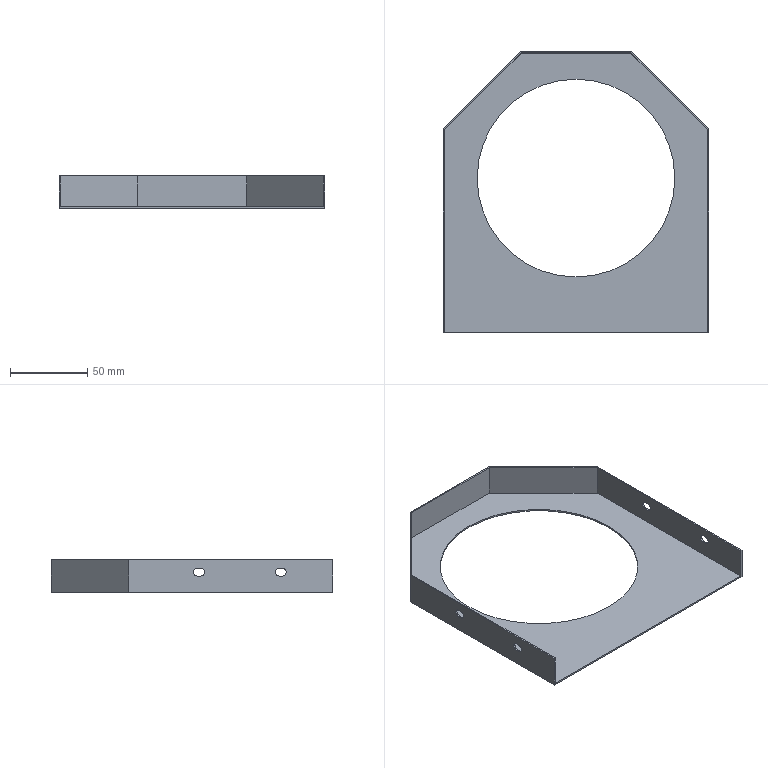Part | SolidWorks | features BaseBody 1 | 1 solid | 32 faces | box 172 x 182 x 21 mm | volume 25333 mm3 | plane 22 | cylinder 10 | commonest cylinder face diameters 5 x8 128 x2
STEP:
#1=CARTESIAN_POINT('',(150.,-82.,1.));
#2=VERTEX_POINT('',#1);
#3=CARTESIAN_POINT('',(22.,-82.,1.));
#4=VERTEX_POINT('',#3);
#5=CARTESIAN_POINT('',(86.,-82.,1.));
#6=DIRECTION('',(0.,0.,-1.));
#7=DIRECTION('',(-1.,0.,0.));
#8=AXIS2_PLACEMENT_3D('',#5,#6,#7);
#9=CIRCLE('',#8,64.);
#10=EDGE_CURVE('',#2,#4,#9,.T.);
#11=ORIENTED_EDGE('',*,*,#10,.F.);
#12=CARTESIAN_POINT('',(150.,-82.,0.));
#13=VERTEX_POINT('',#12);
#14=CARTESIAN_POINT('',(150.,-82.,1.));
#15=DIRECTION('',(0.,0.,-1.));
#16=VECTOR('',#15,1000.);
#17=LINE('',#14,#16);
#18=EDGE_CURVE('',#2,#13,#17,.T.);
#19=ORIENTED_EDGE('',*,*,#18,.T.);
#20=CARTESIAN_POINT('',(22.,-82.,0.));
#21=VERTEX_POINT('',#20);
#22=CARTESIAN_POINT('',(86.,-82.,0.));
#23=DIRECTION('',(0.,0.,-1.));
#24=DIRECTION('',(-1.,0.,0.));
#25=AXIS2_PLACEMENT_3D('',#22,#23,#24);
#26=CIRCLE('',#25,64.);
#27=EDGE_CURVE('',#13,#21,#26,.T.);
#28=ORIENTED_EDGE('',*,*,#27,.T.);
#29=CARTESIAN_POINT('',(22.,-82.,1.));
#30=DIRECTION('',(0.,0.,-1.));
#31=VECTOR('',#30,1000.);
#32=LINE('',#29,#31);
#33=EDGE_CURVE('',#4,#21,#32,.T.);
#34=ORIENTED_EDGE('',*,*,#33,.F.);
#35=EDGE_LOOP('',(#11,#19,#28,#34));
#36=FACE_OUTER_BOUND('',#35,.T.);
#37=CARTESIAN_POINT('',(86.,-82.,1.));
#38=DIRECTION('',(0.,0.,-1.));
#39=DIRECTION('',(-1.,0.,0.));
#40=AXIS2_PLACEMENT_3D('',#37,#38,#39);
#41=CYLINDRICAL_SURFACE('',#40,64.);
#42=ADVANCED_FACE('',(#36),#41,.F.);
#43=CARTESIAN_POINT('',(86.,-82.,0.));
#44=DIRECTION('',(0.,0.,-1.));
#45=DIRECTION('',(-1.,0.,0.));
#46=AXIS2_PLACEMENT_3D('',#43,#44,#45);
#47=CIRCLE('',#46,64.);
#48=EDGE_CURVE('',#21,#13,#47,.T.);
#49=ORIENTED_EDGE('',*,*,#48,.F.);
#50=ORIENTED_EDGE('',*,*,#27,.F.);
#51=EDGE_LOOP('',(#49,#50));
#52=FACE_BOUND('',#51,.T.);
#53=CARTESIAN_POINT('',(0.,-182.,0.));
#54=VERTEX_POINT('',#53);
#55=CARTESIAN_POINT('',(172.,-182.,0.));
#56=VERTEX_POINT('',#55);
#57=CARTESIAN_POINT('',(0.,-182.,0.));
#58=DIRECTION('',(1.,0.,0.));
#59=VECTOR('',#58,1000.);
#60=LINE('',#57,#59);
#61=EDGE_CURVE('',#54,#56,#60,.T.);
#62=ORIENTED_EDGE('',*,*,#61,.F.);
#63=CARTESIAN_POINT('',(0.,-50.,0.));
#64=VERTEX_POINT('',#63);
#65=CARTESIAN_POINT('',(0.,0.,0.));
#66=DIRECTION('',(0.,-1.,0.));
#67=VECTOR('',#66,1000.);
#68=LINE('',#65,#67);
#69=EDGE_CURVE('',#64,#54,#68,.T.);
#70=ORIENTED_EDGE('',*,*,#69,.F.);
#71=CARTESIAN_POINT('',(50.,0.,0.));
#72=VERTEX_POINT('',#71);
#73=CARTESIAN_POINT('',(50.,0.,0.));
#74=DIRECTION('',(-0.7071,-0.7071,0.));
#75=VECTOR('',#74,1000.);
#76=LINE('',#73,#75);
#77=EDGE_CURVE('',#72,#64,#76,.T.);
#78=ORIENTED_EDGE('',*,*,#77,.F.);
#79=CARTESIAN_POINT('',(122.,0.,0.));
#80=VERTEX_POINT('',#79);
#81=CARTESIAN_POINT('',(0.,0.,0.));
#82=DIRECTION('',(-1.,0.,0.));
#83=VECTOR('',#82,1000.);
#84=LINE('',#81,#83);
#85=EDGE_CURVE('',#80,#72,#84,.T.);
#86=ORIENTED_EDGE('',*,*,#85,.F.);
#87=CARTESIAN_POINT('',(172.,-50.,0.));
#88=VERTEX_POINT('',#87);
#89=CARTESIAN_POINT('',(172.,-50.,0.));
#90=DIRECTION('',(-0.7071,0.7071,0.));
#91=VECTOR('',#90,1000.);
#92=LINE('',#89,#91);
#93=EDGE_CURVE('',#88,#80,#92,.T.);
#94=ORIENTED_EDGE('',*,*,#93,.F.);
#95=CARTESIAN_POINT('',(172.,0.,0.));
#96=DIRECTION('',(0.,1.,0.));
#97=VECTOR('',#96,1000.);
#98=LINE('',#95,#97);
#99=EDGE_CURVE('',#56,#88,#98,.T.);
#100=ORIENTED_EDGE('',*,*,#99,.F.);
#101=EDGE_LOOP('',(#62,#70,#78,#86,#94,#100));
#102=FACE_OUTER_BOUND('',#101,.T.);
#103=CARTESIAN_POINT('',(0.,0.,0.));
#104=DIRECTION('',(0.,0.,1.));
#105=DIRECTION('',(1.,0.,0.));
#106=AXIS2_PLACEMENT_3D('',#103,#104,#105);
#107=PLANE('',#106);
#108=ADVANCED_FACE('',(#52,#102),#107,.F.);
#109=ORIENTED_EDGE('',*,*,#18,.F.);
#110=CARTESIAN_POINT('',(86.,-82.,1.));
#111=DIRECTION('',(0.,0.,-1.));
#112=DIRECTION('',(-1.,0.,0.));
#113=AXIS2_PLACEMENT_3D('',#110,#111,#112);
#114=CIRCLE('',#113,64.);
#115=EDGE_CURVE('',#4,#2,#114,.T.);
#116=ORIENTED_EDGE('',*,*,#115,.F.);
#117=ORIENTED_EDGE('',*,*,#33,.T.);
#118=ORIENTED_EDGE('',*,*,#48,.T.);
#119=EDGE_LOOP('',(#109,#116,#117,#118));
#120=FACE_OUTER_BOUND('',#119,.T.);
#121=CARTESIAN_POINT('',(86.,-82.,1.));
#122=DIRECTION('',(0.,0.,-1.));
#123=DIRECTION('',(-1.,0.,0.));
#124=AXIS2_PLACEMENT_3D('',#121,#122,#123);
#125=CYLINDRICAL_SURFACE('',#124,64.);
#126=ADVANCED_FACE('',(#120),#125,.F.);
#127=CARTESIAN_POINT('',(172.,-94.5,10.5));
#128=VERTEX_POINT('',#127);
#129=CARTESIAN_POINT('',(172.,-94.5,15.5));
#130=VERTEX_POINT('',#129);
#131=CARTESIAN_POINT('',(172.,-94.5,13.));
#132=DIRECTION('',(1.,0.,0.));
#133=DIRECTION('',(0.,0.,1.));
#134=AXIS2_PLACEMENT_3D('',#131,#132,#133);
#135=CIRCLE('',#134,2.5);
#136=EDGE_CURVE('',#128,#130,#135,.T.);
#137=ORIENTED_EDGE('',*,*,#136,.F.);
#138=CARTESIAN_POINT('',(172.,-96.5,10.5));
#139=VERTEX_POINT('',#138);
#140=CARTESIAN_POINT('',(172.,-50.,10.5));
#141=DIRECTION('',(0.,1.,0.));
#142=VECTOR('',#141,1000.);
#143=LINE('',#140,#142);
#144=EDGE_CURVE('',#139,#128,#143,.T.);
#145=ORIENTED_EDGE('',*,*,#144,.F.);
#146=CARTESIAN_POINT('',(172.,-96.5,15.5));
#147=VERTEX_POINT('',#146);
#148=CARTESIAN_POINT('',(172.,-96.5,13.));
#149=DIRECTION('',(1.,0.,0.));
#150=DIRECTION('',(0.,0.,1.));
#151=AXIS2_PLACEMENT_3D('',#148,#149,#150);
#152=CIRCLE('',#151,2.5);
#153=EDGE_CURVE('',#147,#139,#152,.T.);
#154=ORIENTED_EDGE('',*,*,#153,.F.);
#155=CARTESIAN_POINT('',(172.,-50.,15.5));
#156=DIRECTION('',(0.,-1.,0.));
#157=VECTOR('',#156,1000.);
#158=LINE('',#155,#157);
#159=EDGE_CURVE('',#130,#147,#158,.T.);
#160=ORIENTED_EDGE('',*,*,#159,.F.);
#161=EDGE_LOOP('',(#137,#145,#154,#160));
#162=FACE_BOUND('',#161,.T.);
#163=CARTESIAN_POINT('',(172.,-147.5,10.5));
#164=VERTEX_POINT('',#163);
#165=CARTESIAN_POINT('',(172.,-147.5,15.5));
#166=VERTEX_POINT('',#165);
#167=CARTESIAN_POINT('',(172.,-147.5,13.));
#168=DIRECTION('',(1.,0.,0.));
#169=DIRECTION('',(0.,0.,1.));
#170=AXIS2_PLACEMENT_3D('',#167,#168,#169);
#171=CIRCLE('',#170,2.5);
#172=EDGE_CURVE('',#164,#166,#171,.T.);
#173=ORIENTED_EDGE('',*,*,#172,.F.);
#174=CARTESIAN_POINT('',(172.,-149.5,10.5));
#175=VERTEX_POINT('',#174);
#176=CARTESIAN_POINT('',(172.,-50.,10.5));
#177=DIRECTION('',(0.,1.,0.));
#178=VECTOR('',#177,1000.);
#179=LINE('',#176,#178);
#180=EDGE_CURVE('',#175,#164,#179,.T.);
#181=ORIENTED_EDGE('',*,*,#180,.F.);
#182=CARTESIAN_POINT('',(172.,-149.5,15.5));
#183=VERTEX_POINT('',#182);
#184=CARTESIAN_POINT('',(172.,-149.5,13.));
#185=DIRECTION('',(1.,0.,0.));
#186=DIRECTION('',(0.,0.,1.));
#187=AXIS2_PLACEMENT_3D('',#184,#185,#186);
#188=CIRCLE('',#187,2.5);
#189=EDGE_CURVE('',#183,#175,#188,.T.);
#190=ORIENTED_EDGE('',*,*,#189,.F.);
#191=CARTESIAN_POINT('',(172.,-50.,15.5));
#192=DIRECTION('',(0.,-1.,0.));
#193=VECTOR('',#192,1000.);
#194=LINE('',#191,#193);
#195=EDGE_CURVE('',#166,#183,#194,.T.);
#196=ORIENTED_EDGE('',*,*,#195,.F.);
#197=EDGE_LOOP('',(#173,#181,#190,#196));
#198=FACE_BOUND('',#197,.T.);
#199=CARTESIAN_POINT('',(172.,-50.,21.));
#200=VERTEX_POINT('',#199);
#201=CARTESIAN_POINT('',(172.,-50.,1.));
#202=DIRECTION('',(0.,0.,-1.));
#203=VECTOR('',#202,1000.);
#204=LINE('',#201,#203);
#205=EDGE_CURVE('',#200,#88,#204,.T.);
#206=ORIENTED_EDGE('',*,*,#205,.F.);
#207=CARTESIAN_POINT('',(172.,-182.,21.));
#208=VERTEX_POINT('',#207);
#209=CARTESIAN_POINT('',(172.,-50.,21.));
#210=DIRECTION('',(0.,1.,0.));
#211=VECTOR('',#210,1000.);
#212=LINE('',#209,#211);
#213=EDGE_CURVE('',#208,#200,#212,.T.);
#214=ORIENTED_EDGE('',*,*,#213,.F.);
#215=CARTESIAN_POINT('',(172.,-182.,1.));
#216=DIRECTION('',(0.,0.,1.));
#217=VECTOR('',#216,1000.);
#218=LINE('',#215,#217);
#219=EDGE_CURVE('',#56,#208,#218,.T.);
#220=ORIENTED_EDGE('',*,*,#219,.F.);
#221=ORIENTED_EDGE('',*,*,#99,.T.);
#222=EDGE_LOOP('',(#206,#214,#220,#221));
#223=FACE_OUTER_BOUND('',#222,.T.);
#224=CARTESIAN_POINT('',(172.,-50.,1.));
#225=DIRECTION('',(-1.,0.,0.));
#226=DIRECTION('',(0.,-1.,0.));
#227=AXIS2_PLACEMENT_3D('',#224,#225,#226);
#228=PLANE('',#227);
#229=ADVANCED_FACE('',(#162,#198,#223),#228,.F.);
#230=ORIENTED_EDGE('',*,*,#219,.T.);
#231=CARTESIAN_POINT('',(171.,-182.,21.));
#232=VERTEX_POINT('',#231);
#233=CARTESIAN_POINT('',(0.,-182.,21.));
#234=DIRECTION('',(1.,0.,0.));
#235=VECTOR('',#234,1000.);
#236=LINE('',#233,#235);
#237=EDGE_CURVE('',#232,#208,#236,.T.);
#238=ORIENTED_EDGE('',*,*,#237,.F.);
#239=CARTESIAN_POINT('',(171.,-182.,1.));
#240=VERTEX_POINT('',#239);
#241=CARTESIAN_POINT('',(171.,-182.,1.));
#242=DIRECTION('',(0.,0.,1.));
#243=VECTOR('',#242,1000.);
#244=LINE('',#241,#243);
#245=EDGE_CURVE('',#240,#232,#244,.T.);
#246=ORIENTED_EDGE('',*,*,#245,.F.);
#247=CARTESIAN_POINT('',(1.,-182.,1.));
#248=VERTEX_POINT('',#247);
#249=CARTESIAN_POINT('',(0.,-182.,1.));
#250=DIRECTION('',(1.,0.,0.));
#251=VECTOR('',#250,1000.);
#252=LINE('',#249,#251);
#253=EDGE_CURVE('',#248,#240,#252,.T.);
#254=ORIENTED_EDGE('',*,*,#253,.F.);
#255=CARTESIAN_POINT('',(1.,-182.,21.));
#256=VERTEX_POINT('',#255);
#257=CARTESIAN_POINT('',(1.,-182.,1.));
#258=DIRECTION('',(0.,0.,-1.));
#259=VECTOR('',#258,1000.);
#260=LINE('',#257,#259);
#261=EDGE_CURVE('',#256,#248,#260,.T.);
#262=ORIENTED_EDGE('',*,*,#261,.F.);
#263=CARTESIAN_POINT('',(0.,-182.,21.));
#264=VERTEX_POINT('',#263);
#265=CARTESIAN_POINT('',(0.,-182.,21.));
#266=DIRECTION('',(1.,0.,0.));
#267=VECTOR('',#266,1000.);
#268=LINE('',#265,#267);
#269=EDGE_CURVE('',#264,#256,#268,.T.);
#270=ORIENTED_EDGE('',*,*,#269,.F.);
#271=CARTESIAN_POINT('',(0.,-182.,1.));
#272=DIRECTION('',(0.,0.,1.));
#273=VECTOR('',#272,1000.);
#274=LINE('',#271,#273);
#275=EDGE_CURVE('',#54,#264,#274,.T.);
#276=ORIENTED_EDGE('',*,*,#275,.F.);
#277=ORIENTED_EDGE('',*,*,#61,.T.);
#278=EDGE_LOOP('',(#230,#238,#246,#254,#262,#270,#276,#277));
#279=FACE_OUTER_BOUND('',#278,.T.);
#280=CARTESIAN_POINT('',(0.,-182.,1.));
#281=DIRECTION('',(0.,1.,0.));
#282=DIRECTION('',(0.,0.,1.));
#283=AXIS2_PLACEMENT_3D('',#280,#281,#282);
#284=PLANE('',#283);
#285=ADVANCED_FACE('',(#279),#284,.F.);
#286=CARTESIAN_POINT('',(0.,-94.5,15.5));
#287=VERTEX_POINT('',#286);
#288=CARTESIAN_POINT('',(0.,-94.5,10.5));
#289=VERTEX_POINT('',#288);
#290=CARTESIAN_POINT('',(0.,-94.5,13.));
#291=DIRECTION('',(-1.,0.,0.));
#292=DIRECTION('',(0.,0.,1.));
#293=AXIS2_PLACEMENT_3D('',#290,#291,#292);
#294=CIRCLE('',#293,2.5);
#295=EDGE_CURVE('',#287,#289,#294,.T.);
#296=ORIENTED_EDGE('',*,*,#295,.F.);
#297=CARTESIAN_POINT('',(0.,-96.5,15.5));
#298=VERTEX_POINT('',#297);
#299=CARTESIAN_POINT('',(0.,-50.,15.5));
#300=DIRECTION('',(0.,1.,0.));
#301=VECTOR('',#300,1000.);
#302=LINE('',#299,#301);
#303=EDGE_CURVE('',#298,#287,#302,.T.);
#304=ORIENTED_EDGE('',*,*,#303,.F.);
#305=CARTESIAN_POINT('',(0.,-96.5,10.5));
#306=VERTEX_POINT('',#305);
#307=CARTESIAN_POINT('',(0.,-96.5,13.));
#308=DIRECTION('',(-1.,0.,0.));
#309=DIRECTION('',(0.,0.,1.));
#310=AXIS2_PLACEMENT_3D('',#307,#308,#309);
#311=CIRCLE('',#310,2.5);
#312=EDGE_CURVE('',#306,#298,#311,.T.);
#313=ORIENTED_EDGE('',*,*,#312,.F.);
#314=CARTESIAN_POINT('',(0.,-50.,10.5));
#315=DIRECTION('',(0.,-1.,0.));
#316=VECTOR('',#315,1000.);
#317=LINE('',#314,#316);
#318=EDGE_CURVE('',#289,#306,#317,.T.);
#319=ORIENTED_EDGE('',*,*,#318,.F.);
#320=EDGE_LOOP('',(#296,#304,#313,#319));
#321=FACE_BOUND('',#320,.T.);
#322=CARTESIAN_POINT('',(0.,-147.5,15.5));
#323=VERTEX_POINT('',#322);
#324=CARTESIAN_POINT('',(0.,-147.5,10.5));
#325=VERTEX_POINT('',#324);
#326=CARTESIAN_POINT('',(0.,-147.5,13.));
#327=DIRECTION('',(-1.,0.,0.));
#328=DIRECTION('',(0.,0.,1.));
#329=AXIS2_PLACEMENT_3D('',#326,#327,#328);
#330=CIRCLE('',#329,2.5);
#331=EDGE_CURVE('',#323,#325,#330,.T.);
#332=ORIENTED_EDGE('',*,*,#331,.F.);
#333=CARTESIAN_POINT('',(0.,-149.5,15.5));
#334=VERTEX_POINT('',#333);
#335=CARTESIAN_POINT('',(0.,-50.,15.5));
#336=DIRECTION('',(0.,1.,0.));
#337=VECTOR('',#336,1000.);
#338=LINE('',#335,#337);
#339=EDGE_CURVE('',#334,#323,#338,.T.);
#340=ORIENTED_EDGE('',*,*,#339,.F.);
#341=CARTESIAN_POINT('',(0.,-149.5,10.5));
#342=VERTEX_POINT('',#341);
#343=CARTESIAN_POINT('',(0.,-149.5,13.));
#344=DIRECTION('',(-1.,0.,0.));
#345=DIRECTION('',(0.,0.,1.));
#346=AXIS2_PLACEMENT_3D('',#343,#344,#345);
#347=CIRCLE('',#346,2.5);
#348=EDGE_CURVE('',#342,#334,#347,.T.);
#349=ORIENTED_EDGE('',*,*,#348,.F.);
#350=CARTESIAN_POINT('',(0.,-50.,10.5));
#351=DIRECTION('',(0.,-1.,0.));
#352=VECTOR('',#351,1000.);
#353=LINE('',#350,#352);
#354=EDGE_CURVE('',#325,#342,#353,.T.);
#355=ORIENTED_EDGE('',*,*,#354,.F.);
#356=EDGE_LOOP('',(#332,#340,#349,#355));
#357=FACE_BOUND('',#356,.T.);
#358=ORIENTED_EDGE('',*,*,#275,.T.);
#359=CARTESIAN_POINT('',(0.,-50.,21.));
#360=VERTEX_POINT('',#359);
#361=CARTESIAN_POINT('',(0.,-50.,21.));
#362=DIRECTION('',(0.,-1.,0.));
#363=VECTOR('',#362,1000.);
#364=LINE('',#361,#363);
#365=EDGE_CURVE('',#360,#264,#364,.T.);
#366=ORIENTED_EDGE('',*,*,#365,.F.);
#367=CARTESIAN_POINT('',(0.,-50.,1.));
#368=DIRECTION('',(0.,0.,1.));
#369=VECTOR('',#368,1000.);
#370=LINE('',#367,#369);
#371=EDGE_CURVE('',#64,#360,#370,.T.);
#372=ORIENTED_EDGE('',*,*,#371,.F.);
#373=ORIENTED_EDGE('',*,*,#69,.T.);
#374=EDGE_LOOP('',(#358,#366,#372,#373));
#375=FACE_OUTER_BOUND('',#374,.T.);
#376=CARTESIAN_POINT('',(0.,-50.,1.));
#377=DIRECTION('',(1.,0.,0.));
#378=DIRECTION('',(0.,1.,0.));
#379=AXIS2_PLACEMENT_3D('',#376,#377,#378);
#380=PLANE('',#379);
#381=ADVANCED_FACE('',(#321,#357,#375),#380,.F.);
#382=ORIENTED_EDGE('',*,*,#371,.T.);
#383=CARTESIAN_POINT('',(50.,0.,21.));
#384=VERTEX_POINT('',#383);
#385=CARTESIAN_POINT('',(0.,-50.,21.));
#386=DIRECTION('',(-0.7071,-0.7071,0.));
#387=VECTOR('',#386,1000.);
#388=LINE('',#385,#387);
#389=EDGE_CURVE('',#384,#360,#388,.T.);
#390=ORIENTED_EDGE('',*,*,#389,.F.);
#391=CARTESIAN_POINT('',(50.,0.,1.));
#392=DIRECTION('',(0.,0.,1.));
#393=VECTOR('',#392,1000.);
#394=LINE('',#391,#393);
#395=EDGE_CURVE('',#72,#384,#394,.T.);
#396=ORIENTED_EDGE('',*,*,#395,.F.);
#397=ORIENTED_EDGE('',*,*,#77,.T.);
#398=EDGE_LOOP('',(#382,#390,#396,#397));
#399=FACE_OUTER_BOUND('',#398,.T.);
#400=CARTESIAN_POINT('',(0.,-50.,1.));
#401=DIRECTION('',(0.7071,-0.7071,0.));
#402=DIRECTION('',(0.7071,0.7071,0.));
#403=AXIS2_PLACEMENT_3D('',#400,#401,#402);
#404=PLANE('',#403);
#405=ADVANCED_FACE('',(#399),#404,.F.);
#406=ORIENTED_EDGE('',*,*,#395,.T.);
#407=CARTESIAN_POINT('',(122.,0.,21.));
#408=VERTEX_POINT('',#407);
#409=CARTESIAN_POINT('',(50.,0.,21.));
#410=DIRECTION('',(-1.,0.,0.));
#411=VECTOR('',#410,1000.);
#412=LINE('',#409,#411);
#413=EDGE_CURVE('',#408,#384,#412,.T.);
#414=ORIENTED_EDGE('',*,*,#413,.F.);
#415=CARTESIAN_POINT('',(122.,0.,1.));
#416=DIRECTION('',(0.,0.,1.));
#417=VECTOR('',#416,1000.);
#418=LINE('',#415,#417);
#419=EDGE_CURVE('',#80,#408,#418,.T.);
#420=ORIENTED_EDGE('',*,*,#419,.F.);
#421=ORIENTED_EDGE('',*,*,#85,.T.);
#422=EDGE_LOOP('',(#406,#414,#420,#421));
#423=FACE_OUTER_BOUND('',#422,.T.);
#424=CARTESIAN_POINT('',(50.,0.,1.));
#425=DIRECTION('',(0.,-1.,0.));
#426=DIRECTION('',(0.,0.,-1.));
#427=AXIS2_PLACEMENT_3D('',#424,#425,#426);
#428=PLANE('',#427);
#429=ADVANCED_FACE('',(#423),#428,.F.);
#430=ORIENTED_EDGE('',*,*,#419,.T.);
#431=CARTESIAN_POINT('',(122.,0.,21.));
#432=DIRECTION('',(-0.7071,0.7071,0.));
#433=VECTOR('',#432,1000.);
#434=LINE('',#431,#433);
#435=EDGE_CURVE('',#200,#408,#434,.T.);
#436=ORIENTED_EDGE('',*,*,#435,.F.);
#437=ORIENTED_EDGE('',*,*,#205,.T.);
#438=ORIENTED_EDGE('',*,*,#93,.T.);
#439=EDGE_LOOP('',(#430,#436,#437,#438));
#440=FACE_OUTER_BOUND('',#439,.T.);
#441=CARTESIAN_POINT('',(122.,0.,1.));
#442=DIRECTION('',(-0.7071,-0.7071,0.));
#443=DIRECTION('',(0.7071,-0.7071,0.));
#444=AXIS2_PLACEMENT_3D('',#441,#442,#443);
#445=PLANE('',#444);
#446=ADVANCED_FACE('',(#440),#445,.F.);
#447=ORIENTED_EDGE('',*,*,#115,.T.);
#448=ORIENTED_EDGE('',*,*,#10,.T.);
#449=EDGE_LOOP('',(#447,#448));
#450=FACE_BOUND('',#449,.T.);
#451=CARTESIAN_POINT('',(1.,-50.414,1.));
#452=VERTEX_POINT('',#451);
#453=CARTESIAN_POINT('',(1.,0.,1.));
#454=DIRECTION('',(0.,-1.,0.));
#455=VECTOR('',#454,1000.);
#456=LINE('',#453,#455);
#457=EDGE_CURVE('',#452,#248,#456,.T.);
#458=ORIENTED_EDGE('',*,*,#457,.T.);
#459=ORIENTED_EDGE('',*,*,#253,.T.);
#460=CARTESIAN_POINT('',(171.,-50.414,1.));
#461=VERTEX_POINT('',#460);
#462=CARTESIAN_POINT('',(171.,0.,1.));
#463=DIRECTION('',(0.,1.,0.));
#464=VECTOR('',#463,1000.);
#465=LINE('',#462,#464);
#466=EDGE_CURVE('',#240,#461,#465,.T.);
#467=ORIENTED_EDGE('',*,*,#466,.T.);
#468=CARTESIAN_POINT('',(121.586,-1.,1.));
#469=VERTEX_POINT('',#468);
#470=CARTESIAN_POINT('',(171.,-50.414,1.));
#471=DIRECTION('',(-0.7071,0.7071,0.));
#472=VECTOR('',#471,1000.);
#473=LINE('',#470,#472);
#474=EDGE_CURVE('',#461,#469,#473,.T.);
#475=ORIENTED_EDGE('',*,*,#474,.T.);
#476=CARTESIAN_POINT('',(50.414,-1.,1.));
#477=VERTEX_POINT('',#476);
#478=CARTESIAN_POINT('',(0.,-1.,1.));
#479=DIRECTION('',(-1.,0.,0.));
#480=VECTOR('',#479,1000.);
#481=LINE('',#478,#480);
#482=EDGE_CURVE('',#469,#477,#481,.T.);
#483=ORIENTED_EDGE('',*,*,#482,.T.);
#484=CARTESIAN_POINT('',(50.414,-1.,1.));
#485=DIRECTION('',(-0.7071,-0.7071,0.));
#486=VECTOR('',#485,1000.);
#487=LINE('',#484,#486);
#488=EDGE_CURVE('',#477,#452,#487,.T.);
#489=ORIENTED_EDGE('',*,*,#488,.T.);
#490=EDGE_LOOP('',(#458,#459,#467,#475,#483,#489));
#491=FACE_OUTER_BOUND('',#490,.T.);
#492=CARTESIAN_POINT('',(0.,0.,1.));
#493=DIRECTION('',(0.,0.,1.));
#494=DIRECTION('',(1.,0.,0.));
#495=AXIS2_PLACEMENT_3D('',#492,#493,#494);
#496=PLANE('',#495);
#497=ADVANCED_FACE('',(#450,#491),#496,.T.);
#498=ORIENTED_EDGE('',*,*,#159,.T.);
#499=CARTESIAN_POINT('',(171.,-96.5,15.5));
#500=VERTEX_POINT('',#499);
#501=CARTESIAN_POINT('',(172.,-96.5,15.5));
#502=DIRECTION('',(1.,0.,0.));
#503=VECTOR('',#502,1000.);
#504=LINE('',#501,#503);
#505=EDGE_CURVE('',#500,#147,#504,.T.);
#506=ORIENTED_EDGE('',*,*,#505,.F.);
#507=CARTESIAN_POINT('',(171.,-94.5,15.5));
#508=VERTEX_POINT('',#507);
#509=CARTESIAN_POINT('',(171.,-94.5,15.5));
#510=DIRECTION('',(0.,-1.,0.));
#511=VECTOR('',#510,1000.);
#512=LINE('',#509,#511);
#513=EDGE_CURVE('',#508,#500,#512,.T.);
#514=ORIENTED_EDGE('',*,*,#513,.F.);
#515=CARTESIAN_POINT('',(172.,-94.5,15.5));
#516=DIRECTION('',(-1.,0.,0.));
#517=VECTOR('',#516,1000.);
#518=LINE('',#515,#517);
#519=EDGE_CURVE('',#130,#508,#518,.T.);
#520=ORIENTED_EDGE('',*,*,#519,.F.);
#521=EDGE_LOOP('',(#498,#506,#514,#520));
#522=FACE_OUTER_BOUND('',#521,.T.);
#523=CARTESIAN_POINT('',(172.,-94.5,15.5));
#524=DIRECTION('',(0.,0.,1.));
#525=DIRECTION('',(1.,0.,0.));
#526=AXIS2_PLACEMENT_3D('',#523,#524,#525);
#527=PLANE('',#526);
#528=ADVANCED_FACE('',(#522),#527,.F.);
#529=ORIENTED_EDGE('',*,*,#519,.T.);
#530=CARTESIAN_POINT('',(171.,-94.5,10.5));
#531=VERTEX_POINT('',#530);
#532=CARTESIAN_POINT('',(171.,-94.5,13.));
#533=DIRECTION('',(1.,0.,0.));
#534=DIRECTION('',(0.,0.,1.));
#535=AXIS2_PLACEMENT_3D('',#532,#533,#534);
#536=CIRCLE('',#535,2.5);
#537=EDGE_CURVE('',#531,#508,#536,.T.);
#538=ORIENTED_EDGE('',*,*,#537,.F.);
#539=CARTESIAN_POINT('',(172.,-94.5,10.5));
#540=DIRECTION('',(-1.,0.,0.));
#541=VECTOR('',#540,1000.);
#542=LINE('',#539,#541);
#543=EDGE_CURVE('',#128,#531,#542,.T.);
#544=ORIENTED_EDGE('',*,*,#543,.F.);
#545=ORIENTED_EDGE('',*,*,#136,.T.);
#546=EDGE_LOOP('',(#529,#538,#544,#545));
#547=FACE_OUTER_BOUND('',#546,.T.);
#548=CARTESIAN_POINT('',(172.,-94.5,13.));
#549=DIRECTION('',(-1.,0.,0.));
#550=DIRECTION('',(0.,0.,1.));
#551=AXIS2_PLACEMENT_3D('',#548,#549,#550);
#552=CYLINDRICAL_SURFACE('',#551,2.5);
#553=ADVANCED_FACE('',(#547),#552,.F.);
#554=ORIENTED_EDGE('',*,*,#144,.T.);
#555=ORIENTED_EDGE('',*,*,#543,.T.);
#556=CARTESIAN_POINT('',(171.,-96.5,10.5));
#557=VERTEX_POINT('',#556);
#558=CARTESIAN_POINT('',(171.,-94.5,10.5));
#559=DIRECTION('',(0.,1.,0.));
#560=VECTOR('',#559,1000.);
#561=LINE('',#558,#560);
#562=EDGE_CURVE('',#557,#531,#561,.T.);
#563=ORIENTED_EDGE('',*,*,#562,.F.);
#564=CARTESIAN_POINT('',(172.,-96.5,10.5));
#565=DIRECTION('',(-1.,0.,0.));
#566=VECTOR('',#565,1000.);
#567=LINE('',#564,#566);
#568=EDGE_CURVE('',#139,#557,#567,.T.);
#569=ORIENTED_EDGE('',*,*,#568,.F.);
#570=EDGE_LOOP('',(#554,#555,#563,#569));
#571=FACE_OUTER_BOUND('',#570,.T.);
#572=CARTESIAN_POINT('',(172.,-94.5,10.5));
#573=DIRECTION('',(0.,0.,-1.));
#574=DIRECTION('',(-1.,0.,0.));
#575=AXIS2_PLACEMENT_3D('',#572,#573,#574);
#576=PLANE('',#575);
#577=ADVANCED_FACE('',(#571),#576,.F.);
#578=ORIENTED_EDGE('',*,*,#153,.T.);
#579=ORIENTED_EDGE('',*,*,#568,.T.);
#580=CARTESIAN_POINT('',(171.,-96.5,13.));
#581=DIRECTION('',(1.,0.,0.));
#582=DIRECTION('',(0.,0.,1.));
#583=AXIS2_PLACEMENT_3D('',#580,#581,#582);
#584=CIRCLE('',#583,2.5);
#585=EDGE_CURVE('',#500,#557,#584,.T.);
#586=ORIENTED_EDGE('',*,*,#585,.F.);
#587=ORIENTED_EDGE('',*,*,#505,.T.);
#588=EDGE_LOOP('',(#578,#579,#586,#587));
#589=FACE_OUTER_BOUND('',#588,.T.);
#590=CARTESIAN_POINT('',(172.,-96.5,13.));
#591=DIRECTION('',(-1.,0.,0.));
#592=DIRECTION('',(0.,0.,1.));
#593=AXIS2_PLACEMENT_3D('',#590,#591,#592);
#594=CYLINDRICAL_SURFACE('',#593,2.5);
#595=ADVANCED_FACE('',(#589),#594,.F.);
#596=ORIENTED_EDGE('',*,*,#195,.T.);
#597=CARTESIAN_POINT('',(171.,-149.5,15.5));
#598=VERTEX_POINT('',#597);
#599=CARTESIAN_POINT('',(172.,-149.5,15.5));
#600=DIRECTION('',(1.,0.,0.));
#601=VECTOR('',#600,1000.);
#602=LINE('',#599,#601);
#603=EDGE_CURVE('',#598,#183,#602,.T.);
#604=ORIENTED_EDGE('',*,*,#603,.F.);
#605=CARTESIAN_POINT('',(171.,-147.5,15.5));
#606=VERTEX_POINT('',#605);
#607=CARTESIAN_POINT('',(171.,-147.5,15.5));
#608=DIRECTION('',(0.,-1.,0.));
#609=VECTOR('',#608,1000.);
#610=LINE('',#607,#609);
#611=EDGE_CURVE('',#606,#598,#610,.T.);
#612=ORIENTED_EDGE('',*,*,#611,.F.);
#613=CARTESIAN_POINT('',(172.,-147.5,15.5));
#614=DIRECTION('',(-1.,0.,0.));
#615=VECTOR('',#614,1000.);
#616=LINE('',#613,#615);
#617=EDGE_CURVE('',#166,#606,#616,.T.);
#618=ORIENTED_EDGE('',*,*,#617,.F.);
#619=EDGE_LOOP('',(#596,#604,#612,#618));
#620=FACE_OUTER_BOUND('',#619,.T.);
#621=CARTESIAN_POINT('',(172.,-147.5,15.5));
#622=DIRECTION('',(0.,0.,1.));
#623=DIRECTION('',(1.,0.,0.));
#624=AXIS2_PLACEMENT_3D('',#621,#622,#623);
#625=PLANE('',#624);
#626=ADVANCED_FACE('',(#620),#625,.F.);
#627=ORIENTED_EDGE('',*,*,#617,.T.);
#628=CARTESIAN_POINT('',(171.,-147.5,10.5));
#629=VERTEX_POINT('',#628);
#630=CARTESIAN_POINT('',(171.,-147.5,13.));
#631=DIRECTION('',(1.,0.,0.));
#632=DIRECTION('',(0.,0.,1.));
#633=AXIS2_PLACEMENT_3D('',#630,#631,#632);
#634=CIRCLE('',#633,2.5);
#635=EDGE_CURVE('',#629,#606,#634,.T.);
#636=ORIENTED_EDGE('',*,*,#635,.F.);
#637=CARTESIAN_POINT('',(172.,-147.5,10.5));
#638=DIRECTION('',(-1.,0.,0.));
#639=VECTOR('',#638,1000.);
#640=LINE('',#637,#639);
#641=EDGE_CURVE('',#164,#629,#640,.T.);
#642=ORIENTED_EDGE('',*,*,#641,.F.);
#643=ORIENTED_EDGE('',*,*,#172,.T.);
#644=EDGE_LOOP('',(#627,#636,#642,#643));
#645=FACE_OUTER_BOUND('',#644,.T.);
#646=CARTESIAN_POINT('',(172.,-147.5,13.));
#647=DIRECTION('',(-1.,0.,0.));
#648=DIRECTION('',(0.,0.,1.));
#649=AXIS2_PLACEMENT_3D('',#646,#647,#648);
#650=CYLINDRICAL_SURFACE('',#649,2.5);
#651=ADVANCED_FACE('',(#645),#650,.F.);
#652=ORIENTED_EDGE('',*,*,#180,.T.);
#653=ORIENTED_EDGE('',*,*,#641,.T.);
#654=CARTESIAN_POINT('',(171.,-149.5,10.5));
#655=VERTEX_POINT('',#654);
#656=CARTESIAN_POINT('',(171.,-147.5,10.5));
#657=DIRECTION('',(0.,1.,0.));
#658=VECTOR('',#657,1000.);
#659=LINE('',#656,#658);
#660=EDGE_CURVE('',#655,#629,#659,.T.);
#661=ORIENTED_EDGE('',*,*,#660,.F.);
#662=CARTESIAN_POINT('',(172.,-149.5,10.5));
#663=DIRECTION('',(-1.,0.,0.));
#664=VECTOR('',#663,1000.);
#665=LINE('',#662,#664);
#666=EDGE_CURVE('',#175,#655,#665,.T.);
#667=ORIENTED_EDGE('',*,*,#666,.F.);
#668=EDGE_LOOP('',(#652,#653,#661,#667));
#669=FACE_OUTER_BOUND('',#668,.T.);
#670=CARTESIAN_POINT('',(172.,-147.5,10.5));
#671=DIRECTION('',(0.,0.,-1.));
#672=DIRECTION('',(-1.,0.,0.));
#673=AXIS2_PLACEMENT_3D('',#670,#671,#672);
#674=PLANE('',#673);
#675=ADVANCED_FACE('',(#669),#674,.F.);
#676=ORIENTED_EDGE('',*,*,#189,.T.);
#677=ORIENTED_EDGE('',*,*,#666,.T.);
#678=CARTESIAN_POINT('',(171.,-149.5,13.));
#679=DIRECTION('',(1.,0.,0.));
#680=DIRECTION('',(0.,0.,1.));
#681=AXIS2_PLACEMENT_3D('',#678,#679,#680);
#682=CIRCLE('',#681,2.5);
#683=EDGE_CURVE('',#598,#655,#682,.T.);
#684=ORIENTED_EDGE('',*,*,#683,.F.);
#685=ORIENTED_EDGE('',*,*,#603,.T.);
#686=EDGE_LOOP('',(#676,#677,#684,#685));
#687=FACE_OUTER_BOUND('',#686,.T.);
#688=CARTESIAN_POINT('',(172.,-149.5,13.));
#689=DIRECTION('',(-1.,0.,0.));
#690=DIRECTION('',(0.,0.,1.));
#691=AXIS2_PLACEMENT_3D('',#688,#689,#690);
#692=CYLINDRICAL_SURFACE('',#691,2.5);
#693=ADVANCED_FACE('',(#687),#692,.F.);
#694=ORIENTED_EDGE('',*,*,#237,.T.);
#695=ORIENTED_EDGE('',*,*,#213,.T.);
#696=ORIENTED_EDGE('',*,*,#435,.T.);
#697=ORIENTED_EDGE('',*,*,#413,.T.);
#698=ORIENTED_EDGE('',*,*,#389,.T.);
#699=ORIENTED_EDGE('',*,*,#365,.T.);
#700=ORIENTED_EDGE('',*,*,#269,.T.);
#701=CARTESIAN_POINT('',(1.,-50.414,21.));
#702=VERTEX_POINT('',#701);
#703=CARTESIAN_POINT('',(1.,0.,21.));
#704=DIRECTION('',(0.,-1.,0.));
#705=VECTOR('',#704,1000.);
#706=LINE('',#703,#705);
#707=EDGE_CURVE('',#702,#256,#706,.T.);
#708=ORIENTED_EDGE('',*,*,#707,.F.);
#709=CARTESIAN_POINT('',(50.414,-1.,21.));
#710=VERTEX_POINT('',#709);
#711=CARTESIAN_POINT('',(50.414,-1.,21.));
#712=DIRECTION('',(-0.7071,-0.7071,0.));
#713=VECTOR('',#712,1000.);
#714=LINE('',#711,#713);
#715=EDGE_CURVE('',#710,#702,#714,.T.);
#716=ORIENTED_EDGE('',*,*,#715,.F.);
#717=CARTESIAN_POINT('',(121.586,-1.,21.));
#718=VERTEX_POINT('',#717);
#719=CARTESIAN_POINT('',(0.,-1.,21.));
#720=DIRECTION('',(-1.,0.,0.));
#721=VECTOR('',#720,1000.);
#722=LINE('',#719,#721);
#723=EDGE_CURVE('',#718,#710,#722,.T.);
#724=ORIENTED_EDGE('',*,*,#723,.F.);
#725=CARTESIAN_POINT('',(171.,-50.414,21.));
#726=VERTEX_POINT('',#725);
#727=CARTESIAN_POINT('',(171.,-50.414,21.));
#728=DIRECTION('',(-0.7071,0.7071,0.));
#729=VECTOR('',#728,1000.);
#730=LINE('',#727,#729);
#731=EDGE_CURVE('',#726,#718,#730,.T.);
#732=ORIENTED_EDGE('',*,*,#731,.F.);
#733=CARTESIAN_POINT('',(171.,0.,21.));
#734=DIRECTION('',(0.,1.,0.));
#735=VECTOR('',#734,1000.);
#736=LINE('',#733,#735);
#737=EDGE_CURVE('',#232,#726,#736,.T.);
#738=ORIENTED_EDGE('',*,*,#737,.F.);
#739=EDGE_LOOP('',(#694,#695,#696,#697,#698,#699,#700,#708,#716,#724,#732,#738));
#740=FACE_OUTER_BOUND('',#739,.T.);
#741=CARTESIAN_POINT('',(0.,0.,21.));
#742=DIRECTION('',(0.,0.,-1.));
#743=DIRECTION('',(-1.,0.,0.));
#744=AXIS2_PLACEMENT_3D('',#741,#742,#743);
#745=PLANE('',#744);
#746=ADVANCED_FACE('',(#740),#745,.F.);
#747=ORIENTED_EDGE('',*,*,#562,.T.);
#748=ORIENTED_EDGE('',*,*,#537,.T.);
#749=ORIENTED_EDGE('',*,*,#513,.T.);
#750=ORIENTED_EDGE('',*,*,#585,.T.);
#751=EDGE_LOOP('',(#747,#748,#749,#750));
#752=FACE_BOUND('',#751,.T.);
#753=ORIENTED_EDGE('',*,*,#660,.T.);
#754=ORIENTED_EDGE('',*,*,#635,.T.);
#755=ORIENTED_EDGE('',*,*,#611,.T.);
#756=ORIENTED_EDGE('',*,*,#683,.T.);
#757=EDGE_LOOP('',(#753,#754,#755,#756));
#758=FACE_BOUND('',#757,.T.);
#759=ORIENTED_EDGE('',*,*,#245,.T.);
#760=ORIENTED_EDGE('',*,*,#737,.T.);
#761=CARTESIAN_POINT('',(171.,-50.414,21.));
#762=DIRECTION('',(0.,0.,1.));
#763=VECTOR('',#762,1000.);
#764=LINE('',#761,#763);
#765=EDGE_CURVE('',#461,#726,#764,.T.);
#766=ORIENTED_EDGE('',*,*,#765,.F.);
#767=ORIENTED_EDGE('',*,*,#466,.F.);
#768=EDGE_LOOP('',(#759,#760,#766,#767));
#769=FACE_OUTER_BOUND('',#768,.T.);
#770=CARTESIAN_POINT('',(171.,-50.,21.));
#771=DIRECTION('',(1.,0.,0.));
#772=DIRECTION('',(0.,1.,0.));
#773=AXIS2_PLACEMENT_3D('',#770,#771,#772);
#774=PLANE('',#773);
#775=ADVANCED_FACE('',(#752,#758,#769),#774,.F.);
#776=CARTESIAN_POINT('',(1.,-94.5,10.5));
#777=VERTEX_POINT('',#776);
#778=CARTESIAN_POINT('',(1.,-94.5,15.5));
#779=VERTEX_POINT('',#778);
#780=CARTESIAN_POINT('',(1.,-94.5,13.));
#781=DIRECTION('',(1.,0.,0.));
#782=DIRECTION('',(0.,0.,1.));
#783=AXIS2_PLACEMENT_3D('',#780,#781,#782);
#784=CIRCLE('',#783,2.5);
#785=EDGE_CURVE('',#777,#779,#784,.T.);
#786=ORIENTED_EDGE('',*,*,#785,.F.);
#787=CARTESIAN_POINT('',(1.,-96.5,10.5));
#788=VERTEX_POINT('',#787);
#789=CARTESIAN_POINT('',(1.,-182.,10.5));
#790=DIRECTION('',(0.,1.,0.));
#791=VECTOR('',#790,1000.);
#792=LINE('',#789,#791);
#793=EDGE_CURVE('',#788,#777,#792,.T.);
#794=ORIENTED_EDGE('',*,*,#793,.F.);
#795=CARTESIAN_POINT('',(1.,-96.5,15.5));
#796=VERTEX_POINT('',#795);
#797=CARTESIAN_POINT('',(1.,-96.5,13.));
#798=DIRECTION('',(1.,0.,0.));
#799=DIRECTION('',(0.,0.,1.));
#800=AXIS2_PLACEMENT_3D('',#797,#798,#799);
#801=CIRCLE('',#800,2.5);
#802=EDGE_CURVE('',#796,#788,#801,.T.);
#803=ORIENTED_EDGE('',*,*,#802,.F.);
#804=CARTESIAN_POINT('',(1.,-182.,15.5));
#805=DIRECTION('',(0.,-1.,0.));
#806=VECTOR('',#805,1000.);
#807=LINE('',#804,#806);
#808=EDGE_CURVE('',#779,#796,#807,.T.);
#809=ORIENTED_EDGE('',*,*,#808,.F.);
#810=EDGE_LOOP('',(#786,#794,#803,#809));
#811=FACE_BOUND('',#810,.T.);
#812=CARTESIAN_POINT('',(1.,-147.5,10.5));
#813=VERTEX_POINT('',#812);
#814=CARTESIAN_POINT('',(1.,-147.5,15.5));
#815=VERTEX_POINT('',#814);
#816=CARTESIAN_POINT('',(1.,-147.5,13.));
#817=DIRECTION('',(1.,0.,0.));
#818=DIRECTION('',(0.,0.,1.));
#819=AXIS2_PLACEMENT_3D('',#816,#817,#818);
#820=CIRCLE('',#819,2.5);
#821=EDGE_CURVE('',#813,#815,#820,.T.);
#822=ORIENTED_EDGE('',*,*,#821,.F.);
#823=CARTESIAN_POINT('',(1.,-149.5,10.5));
#824=VERTEX_POINT('',#823);
#825=CARTESIAN_POINT('',(1.,-182.,10.5));
#826=DIRECTION('',(0.,1.,0.));
#827=VECTOR('',#826,1000.);
#828=LINE('',#825,#827);
#829=EDGE_CURVE('',#824,#813,#828,.T.);
#830=ORIENTED_EDGE('',*,*,#829,.F.);
#831=CARTESIAN_POINT('',(1.,-149.5,15.5));
#832=VERTEX_POINT('',#831);
#833=CARTESIAN_POINT('',(1.,-149.5,13.));
#834=DIRECTION('',(1.,0.,0.));
#835=DIRECTION('',(0.,0.,1.));
#836=AXIS2_PLACEMENT_3D('',#833,#834,#835);
#837=CIRCLE('',#836,2.5);
#838=EDGE_CURVE('',#832,#824,#837,.T.);
#839=ORIENTED_EDGE('',*,*,#838,.F.);
#840=CARTESIAN_POINT('',(1.,-182.,15.5));
#841=DIRECTION('',(0.,-1.,0.));
#842=VECTOR('',#841,1000.);
#843=LINE('',#840,#842);
#844=EDGE_CURVE('',#815,#832,#843,.T.);
#845=ORIENTED_EDGE('',*,*,#844,.F.);
#846=EDGE_LOOP('',(#822,#830,#839,#845));
#847=FACE_BOUND('',#846,.T.);
#848=CARTESIAN_POINT('',(1.,-50.414,21.));
#849=DIRECTION('',(0.,0.,-1.));
#850=VECTOR('',#849,1000.);
#851=LINE('',#848,#850);
#852=EDGE_CURVE('',#702,#452,#851,.T.);
#853=ORIENTED_EDGE('',*,*,#852,.F.);
#854=ORIENTED_EDGE('',*,*,#707,.T.);
#855=ORIENTED_EDGE('',*,*,#261,.T.);
#856=ORIENTED_EDGE('',*,*,#457,.F.);
#857=EDGE_LOOP('',(#853,#854,#855,#856));
#858=FACE_OUTER_BOUND('',#857,.T.);
#859=CARTESIAN_POINT('',(1.,-182.,21.));
#860=DIRECTION('',(-1.,0.,0.));
#861=DIRECTION('',(0.,-1.,0.));
#862=AXIS2_PLACEMENT_3D('',#859,#860,#861);
#863=PLANE('',#862);
#864=ADVANCED_FACE('',(#811,#847,#858),#863,.F.);
#865=ORIENTED_EDGE('',*,*,#318,.T.);
#866=CARTESIAN_POINT('',(172.,-96.5,10.5));
#867=DIRECTION('',(-1.,0.,0.));
#868=VECTOR('',#867,1000.);
#869=LINE('',#866,#868);
#870=EDGE_CURVE('',#788,#306,#869,.T.);
#871=ORIENTED_EDGE('',*,*,#870,.F.);
#872=ORIENTED_EDGE('',*,*,#793,.T.);
#873=CARTESIAN_POINT('',(172.,-94.5,10.5));
#874=DIRECTION('',(1.,0.,0.));
#875=VECTOR('',#874,1000.);
#876=LINE('',#873,#875);
#877=EDGE_CURVE('',#289,#777,#876,.T.);
#878=ORIENTED_EDGE('',*,*,#877,.F.);
#879=EDGE_LOOP('',(#865,#871,#872,#878));
#880=FACE_OUTER_BOUND('',#879,.T.);
#881=CARTESIAN_POINT('',(172.,-94.5,10.5));
#882=DIRECTION('',(0.,0.,-1.));
#883=DIRECTION('',(-1.,0.,0.));
#884=AXIS2_PLACEMENT_3D('',#881,#882,#883);
#885=PLANE('',#884);
#886=ADVANCED_FACE('',(#880),#885,.F.);
#887=ORIENTED_EDGE('',*,*,#877,.T.);
#888=ORIENTED_EDGE('',*,*,#785,.T.);
#889=CARTESIAN_POINT('',(172.,-94.5,15.5));
#890=DIRECTION('',(1.,0.,0.));
#891=VECTOR('',#890,1000.);
#892=LINE('',#889,#891);
#893=EDGE_CURVE('',#287,#779,#892,.T.);
#894=ORIENTED_EDGE('',*,*,#893,.F.);
#895=ORIENTED_EDGE('',*,*,#295,.T.);
#896=EDGE_LOOP('',(#887,#888,#894,#895));
#897=FACE_OUTER_BOUND('',#896,.T.);
#898=CARTESIAN_POINT('',(172.,-94.5,13.));
#899=DIRECTION('',(-1.,0.,0.));
#900=DIRECTION('',(0.,0.,1.));
#901=AXIS2_PLACEMENT_3D('',#898,#899,#900);
#902=CYLINDRICAL_SURFACE('',#901,2.5);
#903=ADVANCED_FACE('',(#897),#902,.F.);
#904=ORIENTED_EDGE('',*,*,#303,.T.);
#905=ORIENTED_EDGE('',*,*,#893,.T.);
#906=ORIENTED_EDGE('',*,*,#808,.T.);
#907=CARTESIAN_POINT('',(172.,-96.5,15.5));
#908=DIRECTION('',(1.,0.,0.));
#909=VECTOR('',#908,1000.);
#910=LINE('',#907,#909);
#911=EDGE_CURVE('',#298,#796,#910,.T.);
#912=ORIENTED_EDGE('',*,*,#911,.F.);
#913=EDGE_LOOP('',(#904,#905,#906,#912));
#914=FACE_OUTER_BOUND('',#913,.T.);
#915=CARTESIAN_POINT('',(172.,-94.5,15.5));
#916=DIRECTION('',(0.,0.,1.));
#917=DIRECTION('',(1.,0.,0.));
#918=AXIS2_PLACEMENT_3D('',#915,#916,#917);
#919=PLANE('',#918);
#920=ADVANCED_FACE('',(#914),#919,.F.);
#921=ORIENTED_EDGE('',*,*,#911,.T.);
#922=ORIENTED_EDGE('',*,*,#802,.T.);
#923=ORIENTED_EDGE('',*,*,#870,.T.);
#924=ORIENTED_EDGE('',*,*,#312,.T.);
#925=EDGE_LOOP('',(#921,#922,#923,#924));
#926=FACE_OUTER_BOUND('',#925,.T.);
#927=CARTESIAN_POINT('',(172.,-96.5,13.));
#928=DIRECTION('',(-1.,0.,0.));
#929=DIRECTION('',(0.,0.,1.));
#930=AXIS2_PLACEMENT_3D('',#927,#928,#929);
#931=CYLINDRICAL_SURFACE('',#930,2.5);
#932=ADVANCED_FACE('',(#926),#931,.F.);
#933=ORIENTED_EDGE('',*,*,#354,.T.);
#934=CARTESIAN_POINT('',(172.,-149.5,10.5));
#935=DIRECTION('',(-1.,0.,0.));
#936=VECTOR('',#935,1000.);
#937=LINE('',#934,#936);
#938=EDGE_CURVE('',#824,#342,#937,.T.);
#939=ORIENTED_EDGE('',*,*,#938,.F.);
#940=ORIENTED_EDGE('',*,*,#829,.T.);
#941=CARTESIAN_POINT('',(172.,-147.5,10.5));
#942=DIRECTION('',(1.,0.,0.));
#943=VECTOR('',#942,1000.);
#944=LINE('',#941,#943);
#945=EDGE_CURVE('',#325,#813,#944,.T.);
#946=ORIENTED_EDGE('',*,*,#945,.F.);
#947=EDGE_LOOP('',(#933,#939,#940,#946));
#948=FACE_OUTER_BOUND('',#947,.T.);
#949=CARTESIAN_POINT('',(172.,-147.5,10.5));
#950=DIRECTION('',(0.,0.,-1.));
#951=DIRECTION('',(-1.,0.,0.));
#952=AXIS2_PLACEMENT_3D('',#949,#950,#951);
#953=PLANE('',#952);
#954=ADVANCED_FACE('',(#948),#953,.F.);
#955=ORIENTED_EDGE('',*,*,#945,.T.);
#956=ORIENTED_EDGE('',*,*,#821,.T.);
#957=CARTESIAN_POINT('',(172.,-147.5,15.5));
#958=DIRECTION('',(1.,0.,0.));
#959=VECTOR('',#958,1000.);
#960=LINE('',#957,#959);
#961=EDGE_CURVE('',#323,#815,#960,.T.);
#962=ORIENTED_EDGE('',*,*,#961,.F.);
#963=ORIENTED_EDGE('',*,*,#331,.T.);
#964=EDGE_LOOP('',(#955,#956,#962,#963));
#965=FACE_OUTER_BOUND('',#964,.T.);
#966=CARTESIAN_POINT('',(172.,-147.5,13.));
#967=DIRECTION('',(-1.,0.,0.));
#968=DIRECTION('',(0.,0.,1.));
#969=AXIS2_PLACEMENT_3D('',#966,#967,#968);
#970=CYLINDRICAL_SURFACE('',#969,2.5);
#971=ADVANCED_FACE('',(#965),#970,.F.);
#972=ORIENTED_EDGE('',*,*,#339,.T.);
#973=ORIENTED_EDGE('',*,*,#961,.T.);
#974=ORIENTED_EDGE('',*,*,#844,.T.);
#975=CARTESIAN_POINT('',(172.,-149.5,15.5));
#976=DIRECTION('',(1.,0.,0.));
#977=VECTOR('',#976,1000.);
#978=LINE('',#975,#977);
#979=EDGE_CURVE('',#334,#832,#978,.T.);
#980=ORIENTED_EDGE('',*,*,#979,.F.);
#981=EDGE_LOOP('',(#972,#973,#974,#980));
#982=FACE_OUTER_BOUND('',#981,.T.);
#983=CARTESIAN_POINT('',(172.,-147.5,15.5));
#984=DIRECTION('',(0.,0.,1.));
#985=DIRECTION('',(1.,0.,0.));
#986=AXIS2_PLACEMENT_3D('',#983,#984,#985);
#987=PLANE('',#986);
#988=ADVANCED_FACE('',(#982),#987,.F.);
#989=ORIENTED_EDGE('',*,*,#979,.T.);
#990=ORIENTED_EDGE('',*,*,#838,.T.);
#991=ORIENTED_EDGE('',*,*,#938,.T.);
#992=ORIENTED_EDGE('',*,*,#348,.T.);
#993=EDGE_LOOP('',(#989,#990,#991,#992));
#994=FACE_OUTER_BOUND('',#993,.T.);
#995=CARTESIAN_POINT('',(172.,-149.5,13.));
#996=DIRECTION('',(-1.,0.,0.));
#997=DIRECTION('',(0.,0.,1.));
#998=AXIS2_PLACEMENT_3D('',#995,#996,#997);
#999=CYLINDRICAL_SURFACE('',#998,2.5);
#1000=ADVANCED_FACE('',(#994),#999,.F.);
#1001=CARTESIAN_POINT('',(50.414,-1.,21.));
#1002=DIRECTION('',(0.,0.,-1.));
#1003=VECTOR('',#1002,1000.);
#1004=LINE('',#1001,#1003);
#1005=EDGE_CURVE('',#710,#477,#1004,.T.);
#1006=ORIENTED_EDGE('',*,*,#1005,.F.);
#1007=ORIENTED_EDGE('',*,*,#715,.T.);
#1008=ORIENTED_EDGE('',*,*,#852,.T.);
#1009=ORIENTED_EDGE('',*,*,#488,.F.);
#1010=EDGE_LOOP('',(#1006,#1007,#1008,#1009));
#1011=FACE_OUTER_BOUND('',#1010,.T.);
#1012=CARTESIAN_POINT('',(0.7071,-50.707,21.));
#1013=DIRECTION('',(-0.7071,0.7071,0.));
#1014=DIRECTION('',(-0.7071,-0.7071,0.));
#1015=AXIS2_PLACEMENT_3D('',#1012,#1013,#1014);
#1016=PLANE('',#1015);
#1017=ADVANCED_FACE('',(#1011),#1016,.F.);
#1018=CARTESIAN_POINT('',(121.586,-1.,21.));
#1019=DIRECTION('',(0.,0.,-1.));
#1020=VECTOR('',#1019,1000.);
#1021=LINE('',#1018,#1020);
#1022=EDGE_CURVE('',#718,#469,#1021,.T.);
#1023=ORIENTED_EDGE('',*,*,#1022,.F.);
#1024=ORIENTED_EDGE('',*,*,#723,.T.);
#1025=ORIENTED_EDGE('',*,*,#1005,.T.);
#1026=ORIENTED_EDGE('',*,*,#482,.F.);
#1027=EDGE_LOOP('',(#1023,#1024,#1025,#1026));
#1028=FACE_OUTER_BOUND('',#1027,.T.);
#1029=CARTESIAN_POINT('',(50.,-1.,21.));
#1030=DIRECTION('',(0.,1.,0.));
#1031=DIRECTION('',(0.,0.,1.));
#1032=AXIS2_PLACEMENT_3D('',#1029,#1030,#1031);
#1033=PLANE('',#1032);
#1034=ADVANCED_FACE('',(#1028),#1033,.F.);
#1035=ORIENTED_EDGE('',*,*,#765,.T.);
#1036=ORIENTED_EDGE('',*,*,#731,.T.);
#1037=ORIENTED_EDGE('',*,*,#1022,.T.);
#1038=ORIENTED_EDGE('',*,*,#474,.F.);
#1039=EDGE_LOOP('',(#1035,#1036,#1037,#1038));
#1040=FACE_OUTER_BOUND('',#1039,.T.);
#1041=CARTESIAN_POINT('',(121.293,-0.7071,21.));
#1042=DIRECTION('',(0.7071,0.7071,0.));
#1043=DIRECTION('',(-0.7071,0.7071,0.));
#1044=AXIS2_PLACEMENT_3D('',#1041,#1042,#1043);
#1045=PLANE('',#1044);
#1046=ADVANCED_FACE('',(#1040),#1045,.F.);
#1047=CLOSED_SHELL('',(#42,#108,#126,#229,#285,#381,#405,#429,#446,#497,#528,#553,#577,#595,#626,#651,#675,#693,#746,#775,#864,#886,#903,#920,#932,#954,#971,#988,#1000,#1017,#1034,#1046));
#1048=MANIFOLD_SOLID_BREP('',#1047);
#1049=CARTESIAN_POINT('',(0.,0.,0.));
#1050=DIRECTION('',(0.,0.,1.));
#1051=DIRECTION('',(1.,0.,0.));
#1052=AXIS2_PLACEMENT_3D('',#1049,#1050,#1051);
#1053=(LENGTH_UNIT()NAMED_UNIT(*)SI_UNIT(.MILLI.,.METRE.));
#1054=UNCERTAINTY_MEASURE_WITH_UNIT(LENGTH_MEASURE(0.00001),#1053,'','');
#1055=(NAMED_UNIT(*)PLANE_ANGLE_UNIT()SI_UNIT($,.RADIAN.));
#1056=(NAMED_UNIT(*)SI_UNIT($,.STERADIAN.)SOLID_ANGLE_UNIT());
#1057=(GEOMETRIC_REPRESENTATION_CONTEXT(3)GLOBAL_UNCERTAINTY_ASSIGNED_CONTEXT((#1054))GLOBAL_UNIT_ASSIGNED_CONTEXT((#1053,#1055,#1056))REPRESENTATION_CONTEXT('',''));
#1058=ADVANCED_BREP_SHAPE_REPRESENTATION('',(#1048,#1052),#1057);